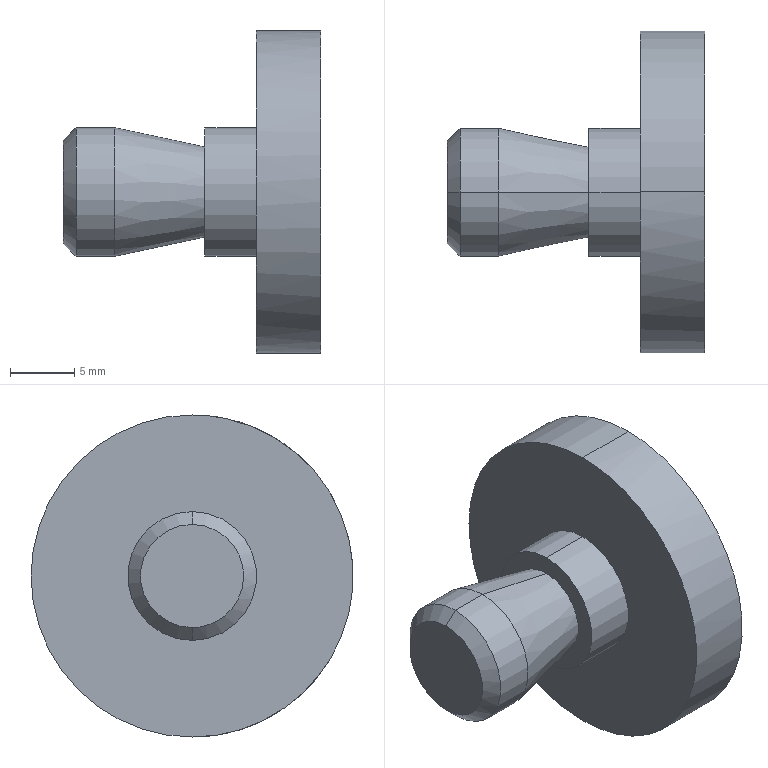Part | STEP file | Positioning_id1786_x_t | 1 solid | 14 faces | box 20 x 25 x 25 mm | volume 3469 mm3 | cylinder 6 | plane 4 | cone 4 | commonest cylinder face diameters 10 x4 25 x2
STEP:
#1=CARTESIAN_POINT('',(0.,0.,0.));
#2=DIRECTION('',(0.,0.,1.));
#3=DIRECTION('',(1.,0.,0.));
#4=AXIS2_PLACEMENT_3D('',#1,#2,#3);
#5=CARTESIAN_POINT('',(-664.,472.5,257.497));
#6=VERTEX_POINT('',#5);
#7=CARTESIAN_POINT('',(-659.,472.5,257.497));
#8=VERTEX_POINT('',#7);
#9=CARTESIAN_POINT('',(-664.,472.5,257.497));
#10=DIRECTION('',(1.,0.,0.));
#11=VECTOR('',#10,1.);
#12=LINE('',#9,#11);
#13=CARTESIAN_POINT('',(-669.,472.5,269.997));
#14=DIRECTION('',(-1.,0.,0.));
#15=DIRECTION('',(0.,0.,-1.));
#16=AXIS2_PLACEMENT_3D('',#13,#14,#15);
#17=CYLINDRICAL_SURFACE('',#16,12.5);
#18=CARTESIAN_POINT('',(6.283,-5.));
#19=DIRECTION('',(0.,-1.));
#20=VECTOR('',#19,1.);
#21=LINE('',#18,#20);
#22=(GEOMETRIC_REPRESENTATION_CONTEXT(2)PARAMETRIC_REPRESENTATION_CONTEXT()REPRESENTATION_CONTEXT('',''));
#23=DEFINITIONAL_REPRESENTATION('',(#21),#22);
#24=PCURVE('',#17,#23);
#25=CARTESIAN_POINT('',(-669.,472.5,269.997));
#26=DIRECTION('',(-1.,0.,0.));
#27=DIRECTION('',(0.,0.,-1.));
#28=AXIS2_PLACEMENT_3D('',#25,#26,#27);
#29=CYLINDRICAL_SURFACE('',#28,12.5);
#30=CARTESIAN_POINT('',(0.,-5.));
#31=DIRECTION('',(0.,-1.));
#32=VECTOR('',#31,1.);
#33=LINE('',#30,#32);
#34=(GEOMETRIC_REPRESENTATION_CONTEXT(2)PARAMETRIC_REPRESENTATION_CONTEXT()REPRESENTATION_CONTEXT('',''));
#35=DEFINITIONAL_REPRESENTATION('',(#33),#34);
#36=PCURVE('',#29,#35);
#37=SURFACE_CURVE('',#12,(#24,#36),.PCURVE_S1.);
#38=EDGE_CURVE('',#6,#8,#37,.T.);
#39=ORIENTED_EDGE('',*,*,#38,.F.);
#40=CARTESIAN_POINT('',(-664.,472.5,282.497));
#41=VERTEX_POINT('',#40);
#42=CARTESIAN_POINT('',(-664.,472.5,269.997));
#43=DIRECTION('',(-1.,0.,0.));
#44=DIRECTION('',(0.,-1.,0.));
#45=AXIS2_PLACEMENT_3D('',#42,#43,#44);
#46=CIRCLE('',#45,12.5);
#47=CARTESIAN_POINT('',(1.571,-5.));
#48=DIRECTION('',(1.,0.));
#49=VECTOR('',#48,1.);
#50=LINE('',#47,#49);
#51=(GEOMETRIC_REPRESENTATION_CONTEXT(2)PARAMETRIC_REPRESENTATION_CONTEXT()REPRESENTATION_CONTEXT('',''));
#52=DEFINITIONAL_REPRESENTATION('',(#50),#51);
#53=PCURVE('',#17,#52);
#54=CARTESIAN_POINT('',(-664.,472.5,269.997));
#55=DIRECTION('',(-1.,0.,0.));
#56=DIRECTION('',(0.,0.,1.));
#57=AXIS2_PLACEMENT_3D('',#54,#55,#56);
#58=PLANE('',#57);
#59=CARTESIAN_POINT('',(0.,0.));
#60=DIRECTION('',(0.,-1.));
#61=AXIS2_PLACEMENT_2D('',#59,#60);
#62=CIRCLE('',#61,12.5);
#63=(GEOMETRIC_REPRESENTATION_CONTEXT(2)PARAMETRIC_REPRESENTATION_CONTEXT()REPRESENTATION_CONTEXT('',''));
#64=DEFINITIONAL_REPRESENTATION('',(#62),#63);
#65=PCURVE('',#58,#64);
#66=SURFACE_CURVE('',#46,(#53,#65),.PCURVE_S1.);
#67=EDGE_CURVE('',#41,#6,#66,.T.);
#68=ORIENTED_EDGE('',*,*,#67,.F.);
#69=CARTESIAN_POINT('',(-659.,472.5,282.497));
#70=VERTEX_POINT('',#69);
#71=CARTESIAN_POINT('',(-664.,472.5,282.497));
#72=DIRECTION('',(-1.,0.,0.));
#73=VECTOR('',#72,1.);
#74=LINE('',#71,#73);
#75=CARTESIAN_POINT('',(3.142,-5.));
#76=DIRECTION('',(0.,1.));
#77=VECTOR('',#76,1.);
#78=LINE('',#75,#77);
#79=(GEOMETRIC_REPRESENTATION_CONTEXT(2)PARAMETRIC_REPRESENTATION_CONTEXT()REPRESENTATION_CONTEXT('',''));
#80=DEFINITIONAL_REPRESENTATION('',(#78),#79);
#81=PCURVE('',#17,#80);
#82=CARTESIAN_POINT('',(3.142,-5.));
#83=DIRECTION('',(0.,1.));
#84=VECTOR('',#83,1.);
#85=LINE('',#82,#84);
#86=(GEOMETRIC_REPRESENTATION_CONTEXT(2)PARAMETRIC_REPRESENTATION_CONTEXT()REPRESENTATION_CONTEXT('',''));
#87=DEFINITIONAL_REPRESENTATION('',(#85),#86);
#88=PCURVE('',#29,#87);
#89=SURFACE_CURVE('',#74,(#81,#88),.PCURVE_S1.);
#90=EDGE_CURVE('',#70,#41,#89,.T.);
#91=ORIENTED_EDGE('',*,*,#90,.F.);
#92=CARTESIAN_POINT('',(-659.,472.5,269.997));
#93=DIRECTION('',(1.,0.,0.));
#94=DIRECTION('',(0.,-1.,0.));
#95=AXIS2_PLACEMENT_3D('',#92,#93,#94);
#96=CIRCLE('',#95,12.5);
#97=CARTESIAN_POINT('',(7.854,-10.));
#98=DIRECTION('',(-1.,0.));
#99=VECTOR('',#98,1.);
#100=LINE('',#97,#99);
#101=(GEOMETRIC_REPRESENTATION_CONTEXT(2)PARAMETRIC_REPRESENTATION_CONTEXT()REPRESENTATION_CONTEXT('',''));
#102=DEFINITIONAL_REPRESENTATION('',(#100),#101);
#103=PCURVE('',#17,#102);
#104=CARTESIAN_POINT('',(-659.,472.5,269.997));
#105=DIRECTION('',(1.,0.,0.));
#106=DIRECTION('',(0.,0.,-1.));
#107=AXIS2_PLACEMENT_3D('',#104,#105,#106);
#108=PLANE('',#107);
#109=CARTESIAN_POINT('',(0.,0.));
#110=DIRECTION('',(0.,-1.));
#111=AXIS2_PLACEMENT_2D('',#109,#110);
#112=CIRCLE('',#111,12.5);
#113=(GEOMETRIC_REPRESENTATION_CONTEXT(2)PARAMETRIC_REPRESENTATION_CONTEXT()REPRESENTATION_CONTEXT('',''));
#114=DEFINITIONAL_REPRESENTATION('',(#112),#113);
#115=PCURVE('',#108,#114);
#116=SURFACE_CURVE('',#96,(#103,#115),.PCURVE_S1.);
#117=EDGE_CURVE('',#8,#70,#116,.T.);
#118=ORIENTED_EDGE('',*,*,#117,.F.);
#119=EDGE_LOOP('',(#39,#68,#91,#118));
#120=FACE_BOUND('',#119,.T.);
#121=ADVANCED_FACE('',(#120),#17,.T.);
#122=CARTESIAN_POINT('',(-664.,472.5,274.997));
#123=VERTEX_POINT('',#122);
#124=CARTESIAN_POINT('',(-664.,472.5,264.997));
#125=VERTEX_POINT('',#124);
#126=CARTESIAN_POINT('',(-664.,472.5,269.997));
#127=DIRECTION('',(-1.,0.,0.));
#128=DIRECTION('',(0.,0.,1.));
#129=AXIS2_PLACEMENT_3D('',#126,#127,#128);
#130=CIRCLE('',#129,5.);
#131=CARTESIAN_POINT('',(0.,0.));
#132=DIRECTION('',(1.,0.));
#133=AXIS2_PLACEMENT_2D('',#131,#132);
#134=CIRCLE('',#133,5.);
#135=(GEOMETRIC_REPRESENTATION_CONTEXT(2)PARAMETRIC_REPRESENTATION_CONTEXT()REPRESENTATION_CONTEXT('',''));
#136=DEFINITIONAL_REPRESENTATION('',(#134),#135);
#137=PCURVE('',#58,#136);
#138=CARTESIAN_POINT('',(-669.,472.5,269.997));
#139=DIRECTION('',(-1.,0.,0.));
#140=DIRECTION('',(0.,0.,-1.));
#141=AXIS2_PLACEMENT_3D('',#138,#139,#140);
#142=CYLINDRICAL_SURFACE('',#141,5.);
#143=CARTESIAN_POINT('',(3.142,-5.));
#144=DIRECTION('',(1.,0.));
#145=VECTOR('',#144,1.);
#146=LINE('',#143,#145);
#147=(GEOMETRIC_REPRESENTATION_CONTEXT(2)PARAMETRIC_REPRESENTATION_CONTEXT()REPRESENTATION_CONTEXT('',''));
#148=DEFINITIONAL_REPRESENTATION('',(#146),#147);
#149=PCURVE('',#142,#148);
#150=SURFACE_CURVE('',#130,(#137,#149),.PCURVE_S1.);
#151=EDGE_CURVE('',#123,#125,#150,.T.);
#152=ORIENTED_EDGE('',*,*,#151,.F.);
#153=CARTESIAN_POINT('',(-664.,472.5,269.997));
#154=DIRECTION('',(-1.,0.,0.));
#155=DIRECTION('',(0.,0.,-1.));
#156=AXIS2_PLACEMENT_3D('',#153,#154,#155);
#157=CIRCLE('',#156,5.);
#158=CARTESIAN_POINT('',(0.,0.));
#159=DIRECTION('',(-1.,0.));
#160=AXIS2_PLACEMENT_2D('',#158,#159);
#161=CIRCLE('',#160,5.);
#162=(GEOMETRIC_REPRESENTATION_CONTEXT(2)PARAMETRIC_REPRESENTATION_CONTEXT()REPRESENTATION_CONTEXT('',''));
#163=DEFINITIONAL_REPRESENTATION('',(#161),#162);
#164=PCURVE('',#58,#163);
#165=CARTESIAN_POINT('',(-669.,472.5,269.997));
#166=DIRECTION('',(-1.,0.,0.));
#167=DIRECTION('',(0.,0.,-1.));
#168=AXIS2_PLACEMENT_3D('',#165,#166,#167);
#169=CYLINDRICAL_SURFACE('',#168,5.);
#170=CARTESIAN_POINT('',(0.,-5.));
#171=DIRECTION('',(1.,0.));
#172=VECTOR('',#171,1.);
#173=LINE('',#170,#172);
#174=(GEOMETRIC_REPRESENTATION_CONTEXT(2)PARAMETRIC_REPRESENTATION_CONTEXT()REPRESENTATION_CONTEXT('',''));
#175=DEFINITIONAL_REPRESENTATION('',(#173),#174);
#176=PCURVE('',#169,#175);
#177=SURFACE_CURVE('',#157,(#164,#176),.PCURVE_S1.);
#178=EDGE_CURVE('',#125,#123,#177,.T.);
#179=ORIENTED_EDGE('',*,*,#178,.F.);
#180=EDGE_LOOP('',(#152,#179));
#181=FACE_BOUND('',#180,.T.);
#182=ORIENTED_EDGE('',*,*,#67,.T.);
#183=CARTESIAN_POINT('',(-664.,472.5,257.497));
#184=CARTESIAN_POINT('',(-664.,460.,257.497));
#185=CARTESIAN_POINT('',(-664.,453.75,269.997));
#186=CARTESIAN_POINT('',(-664.,460.,282.497));
#187=CARTESIAN_POINT('',(-664.,472.5,282.497));
#188=(BOUNDED_CURVE()B_SPLINE_CURVE(4,(#183,#184,#185,#186,#187),.UNSPECIFIED.,.F.,.F.)B_SPLINE_CURVE_WITH_KNOTS((5,5),(0.,1.),.PIECEWISE_BEZIER_KNOTS.)CURVE()GEOMETRIC_REPRESENTATION_ITEM()RATIONAL_B_SPLINE_CURVE((1.,0.7071,0.6667,0.7071,1.))REPRESENTATION_ITEM(''));
#189=CARTESIAN_POINT('',(-12.5,0.));
#190=CARTESIAN_POINT('',(-12.5,-12.5));
#191=CARTESIAN_POINT('',(0.,-18.75));
#192=CARTESIAN_POINT('',(12.5,-12.5));
#193=CARTESIAN_POINT('',(12.5,0.));
#194=(BOUNDED_CURVE()B_SPLINE_CURVE(4,(#189,#190,#191,#192,#193),.UNSPECIFIED.,.F.,.F.)B_SPLINE_CURVE_WITH_KNOTS((5,5),(0.,1.),.PIECEWISE_BEZIER_KNOTS.)CURVE()GEOMETRIC_REPRESENTATION_ITEM()RATIONAL_B_SPLINE_CURVE((1.,0.7071,0.6667,0.7071,1.))REPRESENTATION_ITEM(''));
#195=(GEOMETRIC_REPRESENTATION_CONTEXT(2)PARAMETRIC_REPRESENTATION_CONTEXT()REPRESENTATION_CONTEXT('',''));
#196=DEFINITIONAL_REPRESENTATION('',(#194),#195);
#197=PCURVE('',#58,#196);
#198=CARTESIAN_POINT('',(0.,-5.));
#199=CARTESIAN_POINT('',(0.04285,-5.));
#200=CARTESIAN_POINT('',(0.1297,-5.));
#201=CARTESIAN_POINT('',(0.2633,-5.));
#202=CARTESIAN_POINT('',(0.3999,-5.));
#203=CARTESIAN_POINT('',(0.5394,-5.));
#204=CARTESIAN_POINT('',(0.6816,-5.));
#205=CARTESIAN_POINT('',(0.8261,-5.));
#206=CARTESIAN_POINT('',(0.9725,-5.));
#207=CARTESIAN_POINT('',(1.121,-5.));
#208=CARTESIAN_POINT('',(1.27,-5.));
#209=CARTESIAN_POINT('',(1.42,-5.));
#210=CARTESIAN_POINT('',(1.571,-5.));
#211=CARTESIAN_POINT('',(1.721,-5.));
#212=CARTESIAN_POINT('',(1.872,-5.));
#213=CARTESIAN_POINT('',(2.021,-5.));
#214=CARTESIAN_POINT('',(2.169,-5.));
#215=CARTESIAN_POINT('',(2.316,-5.));
#216=CARTESIAN_POINT('',(2.46,-5.));
#217=CARTESIAN_POINT('',(2.602,-5.));
#218=CARTESIAN_POINT('',(2.742,-5.));
#219=CARTESIAN_POINT('',(2.878,-5.));
#220=CARTESIAN_POINT('',(3.012,-5.));
#221=CARTESIAN_POINT('',(3.099,-5.));
#222=CARTESIAN_POINT('',(3.142,-5.));
#223=B_SPLINE_CURVE_WITH_KNOTS('',3,(#198,#199,#200,#201,#202,#203,#204,#205,#206,#207,#208,#209,#210,#211,#212,#213,#214,#215,#216,#217,#218,#219,#220,#221,#222),.UNSPECIFIED.,.F.,.F.,(4,1,1,1,1,1,1,1,1,1,1,1,1,1,1,1,1,1,1,1,1,1,4),(0.,0.04545,0.09091,0.1364,0.1818,0.2273,0.2727,0.3182,0.3636,0.4091,0.4545,0.5,0.5455,0.5909,0.6364,0.6818,0.7273,0.7727,0.8182,0.8636,0.9091,0.9545,1.),.QUASI_UNIFORM_KNOTS.);
#224=(GEOMETRIC_REPRESENTATION_CONTEXT(2)PARAMETRIC_REPRESENTATION_CONTEXT()REPRESENTATION_CONTEXT('',''));
#225=DEFINITIONAL_REPRESENTATION('',(#223),#224);
#226=PCURVE('',#29,#225);
#227=SURFACE_CURVE('',#188,(#197,#226),.PCURVE_S1.);
#228=EDGE_CURVE('',#6,#41,#227,.T.);
#229=ORIENTED_EDGE('',*,*,#228,.T.);
#230=EDGE_LOOP('',(#182,#229));
#231=FACE_BOUND('',#230,.T.);
#232=ADVANCED_FACE('',(#181,#231),#58,.T.);
#233=CARTESIAN_POINT('',(-659.,472.5,282.497));
#234=CARTESIAN_POINT('',(-659.,460.,282.497));
#235=CARTESIAN_POINT('',(-659.,453.75,269.997));
#236=CARTESIAN_POINT('',(-659.,460.,257.497));
#237=CARTESIAN_POINT('',(-659.,472.5,257.497));
#238=(BOUNDED_CURVE()B_SPLINE_CURVE(4,(#233,#234,#235,#236,#237),.UNSPECIFIED.,.F.,.F.)B_SPLINE_CURVE_WITH_KNOTS((5,5),(0.,1.),.PIECEWISE_BEZIER_KNOTS.)CURVE()GEOMETRIC_REPRESENTATION_ITEM()RATIONAL_B_SPLINE_CURVE((1.,0.7071,0.6667,0.7071,1.))REPRESENTATION_ITEM(''));
#239=CARTESIAN_POINT('',(-12.5,0.));
#240=CARTESIAN_POINT('',(-12.5,-12.5));
#241=CARTESIAN_POINT('',(0.,-18.75));
#242=CARTESIAN_POINT('',(12.5,-12.5));
#243=CARTESIAN_POINT('',(12.5,0.));
#244=(BOUNDED_CURVE()B_SPLINE_CURVE(4,(#239,#240,#241,#242,#243),.UNSPECIFIED.,.F.,.F.)B_SPLINE_CURVE_WITH_KNOTS((5,5),(0.,1.),.PIECEWISE_BEZIER_KNOTS.)CURVE()GEOMETRIC_REPRESENTATION_ITEM()RATIONAL_B_SPLINE_CURVE((1.,0.7071,0.6667,0.7071,1.))REPRESENTATION_ITEM(''));
#245=(GEOMETRIC_REPRESENTATION_CONTEXT(2)PARAMETRIC_REPRESENTATION_CONTEXT()REPRESENTATION_CONTEXT('',''));
#246=DEFINITIONAL_REPRESENTATION('',(#244),#245);
#247=PCURVE('',#108,#246);
#248=CARTESIAN_POINT('',(3.142,-10.));
#249=CARTESIAN_POINT('',(3.099,-10.));
#250=CARTESIAN_POINT('',(3.012,-10.));
#251=CARTESIAN_POINT('',(2.878,-10.));
#252=CARTESIAN_POINT('',(2.742,-10.));
#253=CARTESIAN_POINT('',(2.602,-10.));
#254=CARTESIAN_POINT('',(2.46,-10.));
#255=CARTESIAN_POINT('',(2.316,-10.));
#256=CARTESIAN_POINT('',(2.169,-10.));
#257=CARTESIAN_POINT('',(2.021,-10.));
#258=CARTESIAN_POINT('',(1.872,-10.));
#259=CARTESIAN_POINT('',(1.721,-10.));
#260=CARTESIAN_POINT('',(1.571,-10.));
#261=CARTESIAN_POINT('',(1.42,-10.));
#262=CARTESIAN_POINT('',(1.27,-10.));
#263=CARTESIAN_POINT('',(1.121,-10.));
#264=CARTESIAN_POINT('',(0.9725,-10.));
#265=CARTESIAN_POINT('',(0.8261,-10.));
#266=CARTESIAN_POINT('',(0.6816,-10.));
#267=CARTESIAN_POINT('',(0.5394,-10.));
#268=CARTESIAN_POINT('',(0.3999,-10.));
#269=CARTESIAN_POINT('',(0.2633,-10.));
#270=CARTESIAN_POINT('',(0.1297,-10.));
#271=CARTESIAN_POINT('',(0.04285,-10.));
#272=CARTESIAN_POINT('',(0.,-10.));
#273=B_SPLINE_CURVE_WITH_KNOTS('',3,(#248,#249,#250,#251,#252,#253,#254,#255,#256,#257,#258,#259,#260,#261,#262,#263,#264,#265,#266,#267,#268,#269,#270,#271,#272),.UNSPECIFIED.,.F.,.F.,(4,1,1,1,1,1,1,1,1,1,1,1,1,1,1,1,1,1,1,1,1,1,4),(0.,0.04545,0.09091,0.1364,0.1818,0.2273,0.2727,0.3182,0.3636,0.4091,0.4545,0.5,0.5455,0.5909,0.6364,0.6818,0.7273,0.7727,0.8182,0.8636,0.9091,0.9545,1.),.QUASI_UNIFORM_KNOTS.);
#274=(GEOMETRIC_REPRESENTATION_CONTEXT(2)PARAMETRIC_REPRESENTATION_CONTEXT()REPRESENTATION_CONTEXT('',''));
#275=DEFINITIONAL_REPRESENTATION('',(#273),#274);
#276=PCURVE('',#29,#275);
#277=SURFACE_CURVE('',#238,(#247,#276),.PCURVE_S1.);
#278=EDGE_CURVE('',#70,#8,#277,.T.);
#279=ORIENTED_EDGE('',*,*,#278,.T.);
#280=ORIENTED_EDGE('',*,*,#117,.T.);
#281=EDGE_LOOP('',(#279,#280));
#282=FACE_BOUND('',#281,.T.);
#283=ADVANCED_FACE('',(#282),#108,.T.);
#284=CARTESIAN_POINT('',(-668.,472.5,266.497));
#285=VERTEX_POINT('',#284);
#286=CARTESIAN_POINT('',(-668.,472.5,273.497));
#287=VERTEX_POINT('',#286);
#288=CARTESIAN_POINT('',(-668.,472.5,269.997));
#289=DIRECTION('',(-1.,0.,0.));
#290=DIRECTION('',(0.,0.,-1.));
#291=AXIS2_PLACEMENT_3D('',#288,#289,#290);
#292=CIRCLE('',#291,3.5);
#293=CARTESIAN_POINT('',(-668.,472.5,269.997));
#294=DIRECTION('',(1.,0.,0.));
#295=DIRECTION('',(0.,0.,-1.));
#296=AXIS2_PLACEMENT_3D('',#293,#294,#295);
#297=PLANE('',#296);
#298=CARTESIAN_POINT('',(3.5,0.));
#299=CARTESIAN_POINT('',(3.5,-6.062));
#300=CARTESIAN_POINT('',(-1.75,-3.031));
#301=CARTESIAN_POINT('',(-7.,0.));
#302=CARTESIAN_POINT('',(-1.75,3.031));
#303=CARTESIAN_POINT('',(3.5,6.062));
#304=CARTESIAN_POINT('',(3.5,0.));
#305=(BOUNDED_CURVE()B_SPLINE_CURVE(2,(#298,#299,#300,#301,#302,#303,#304),.UNSPECIFIED.,.T.,.F.)B_SPLINE_CURVE_WITH_KNOTS((1,2,2,2,2,1),(-2.094,0.,2.094,4.189,6.283,8.378),.UNSPECIFIED.)CURVE()GEOMETRIC_REPRESENTATION_ITEM()RATIONAL_B_SPLINE_CURVE((1.,0.5,1.,0.5,1.,0.5,1.))REPRESENTATION_ITEM(''));
#306=(GEOMETRIC_REPRESENTATION_CONTEXT(2)PARAMETRIC_REPRESENTATION_CONTEXT()REPRESENTATION_CONTEXT('',''));
#307=DEFINITIONAL_REPRESENTATION('',(#305),#306);
#308=PCURVE('',#297,#307);
#309=CARTESIAN_POINT('',(-675.,472.5,269.997));
#310=DIRECTION('',(-1.,0.,0.));
#311=DIRECTION('',(0.,0.,1.));
#312=AXIS2_PLACEMENT_3D('',#309,#310,#311);
#313=CONICAL_SURFACE('',#312,5.,0.2111);
#314=CARTESIAN_POINT('',(3.142,-7.));
#315=DIRECTION('',(1.,0.));
#316=VECTOR('',#315,1.);
#317=LINE('',#314,#316);
#318=(GEOMETRIC_REPRESENTATION_CONTEXT(2)PARAMETRIC_REPRESENTATION_CONTEXT()REPRESENTATION_CONTEXT('',''));
#319=DEFINITIONAL_REPRESENTATION('',(#317),#318);
#320=PCURVE('',#313,#319);
#321=SURFACE_CURVE('',#292,(#308,#320),.PCURVE_S1.);
#322=EDGE_CURVE('',#285,#287,#321,.T.);
#323=ORIENTED_EDGE('',*,*,#322,.F.);
#324=CARTESIAN_POINT('',(-668.,472.5,269.997));
#325=DIRECTION('',(-1.,0.,0.));
#326=DIRECTION('',(0.,0.,1.));
#327=AXIS2_PLACEMENT_3D('',#324,#325,#326);
#328=CIRCLE('',#327,3.5);
#329=CARTESIAN_POINT('',(-3.5,0.));
#330=CARTESIAN_POINT('',(-3.5,6.062));
#331=CARTESIAN_POINT('',(1.75,3.031));
#332=CARTESIAN_POINT('',(7.,0.));
#333=CARTESIAN_POINT('',(1.75,-3.031));
#334=CARTESIAN_POINT('',(-3.5,-6.062));
#335=CARTESIAN_POINT('',(-3.5,0.));
#336=(BOUNDED_CURVE()B_SPLINE_CURVE(2,(#329,#330,#331,#332,#333,#334,#335),.UNSPECIFIED.,.T.,.F.)B_SPLINE_CURVE_WITH_KNOTS((1,2,2,2,2,1),(-2.094,0.,2.094,4.189,6.283,8.378),.UNSPECIFIED.)CURVE()GEOMETRIC_REPRESENTATION_ITEM()RATIONAL_B_SPLINE_CURVE((1.,0.5,1.,0.5,1.,0.5,1.))REPRESENTATION_ITEM(''));
#337=(GEOMETRIC_REPRESENTATION_CONTEXT(2)PARAMETRIC_REPRESENTATION_CONTEXT()REPRESENTATION_CONTEXT('',''));
#338=DEFINITIONAL_REPRESENTATION('',(#336),#337);
#339=PCURVE('',#297,#338);
#340=CARTESIAN_POINT('',(-675.,472.5,269.997));
#341=DIRECTION('',(-1.,0.,0.));
#342=DIRECTION('',(0.,0.,1.));
#343=AXIS2_PLACEMENT_3D('',#340,#341,#342);
#344=CONICAL_SURFACE('',#343,5.,0.2111);
#345=CARTESIAN_POINT('',(0.,-7.));
#346=DIRECTION('',(1.,0.));
#347=VECTOR('',#346,1.);
#348=LINE('',#345,#347);
#349=(GEOMETRIC_REPRESENTATION_CONTEXT(2)PARAMETRIC_REPRESENTATION_CONTEXT()REPRESENTATION_CONTEXT('',''));
#350=DEFINITIONAL_REPRESENTATION('',(#348),#349);
#351=PCURVE('',#344,#350);
#352=SURFACE_CURVE('',#328,(#339,#351),.PCURVE_S1.);
#353=EDGE_CURVE('',#287,#285,#352,.T.);
#354=ORIENTED_EDGE('',*,*,#353,.F.);
#355=EDGE_LOOP('',(#323,#354));
#356=FACE_BOUND('',#355,.T.);
#357=CARTESIAN_POINT('',(-668.,472.5,274.997));
#358=VERTEX_POINT('',#357);
#359=CARTESIAN_POINT('',(-668.,472.5,264.997));
#360=VERTEX_POINT('',#359);
#361=CARTESIAN_POINT('',(-668.,472.5,269.997));
#362=DIRECTION('',(1.,0.,0.));
#363=DIRECTION('',(0.,0.,1.));
#364=AXIS2_PLACEMENT_3D('',#361,#362,#363);
#365=CIRCLE('',#364,5.);
#366=CARTESIAN_POINT('',(0.,0.));
#367=DIRECTION('',(-1.,0.));
#368=AXIS2_PLACEMENT_2D('',#366,#367);
#369=CIRCLE('',#368,5.);
#370=(GEOMETRIC_REPRESENTATION_CONTEXT(2)PARAMETRIC_REPRESENTATION_CONTEXT()REPRESENTATION_CONTEXT('',''));
#371=DEFINITIONAL_REPRESENTATION('',(#369),#370);
#372=PCURVE('',#297,#371);
#373=CARTESIAN_POINT('',(3.142,-1.));
#374=DIRECTION('',(-1.,0.));
#375=VECTOR('',#374,1.);
#376=LINE('',#373,#375);
#377=(GEOMETRIC_REPRESENTATION_CONTEXT(2)PARAMETRIC_REPRESENTATION_CONTEXT()REPRESENTATION_CONTEXT('',''));
#378=DEFINITIONAL_REPRESENTATION('',(#376),#377);
#379=PCURVE('',#169,#378);
#380=SURFACE_CURVE('',#365,(#372,#379),.PCURVE_S1.);
#381=EDGE_CURVE('',#358,#360,#380,.T.);
#382=ORIENTED_EDGE('',*,*,#381,.F.);
#383=CARTESIAN_POINT('',(-668.,472.5,269.997));
#384=DIRECTION('',(1.,0.,0.));
#385=DIRECTION('',(0.,0.,-1.));
#386=AXIS2_PLACEMENT_3D('',#383,#384,#385);
#387=CIRCLE('',#386,5.);
#388=CARTESIAN_POINT('',(0.,0.));
#389=DIRECTION('',(1.,0.));
#390=AXIS2_PLACEMENT_2D('',#388,#389);
#391=CIRCLE('',#390,5.);
#392=(GEOMETRIC_REPRESENTATION_CONTEXT(2)PARAMETRIC_REPRESENTATION_CONTEXT()REPRESENTATION_CONTEXT('',''));
#393=DEFINITIONAL_REPRESENTATION('',(#391),#392);
#394=PCURVE('',#297,#393);
#395=CARTESIAN_POINT('',(6.283,-1.));
#396=DIRECTION('',(-1.,0.));
#397=VECTOR('',#396,1.);
#398=LINE('',#395,#397);
#399=(GEOMETRIC_REPRESENTATION_CONTEXT(2)PARAMETRIC_REPRESENTATION_CONTEXT()REPRESENTATION_CONTEXT('',''));
#400=DEFINITIONAL_REPRESENTATION('',(#398),#399);
#401=PCURVE('',#142,#400);
#402=SURFACE_CURVE('',#387,(#394,#401),.PCURVE_S1.);
#403=EDGE_CURVE('',#360,#358,#402,.T.);
#404=ORIENTED_EDGE('',*,*,#403,.F.);
#405=EDGE_LOOP('',(#382,#404));
#406=FACE_BOUND('',#405,.T.);
#407=ADVANCED_FACE('',(#356,#406),#297,.F.);
#408=CARTESIAN_POINT('',(-668.,472.5,264.997));
#409=DIRECTION('',(1.,0.,0.));
#410=VECTOR('',#409,1.);
#411=LINE('',#408,#410);
#412=CARTESIAN_POINT('',(6.283,-1.));
#413=DIRECTION('',(0.,-1.));
#414=VECTOR('',#413,1.);
#415=LINE('',#412,#414);
#416=(GEOMETRIC_REPRESENTATION_CONTEXT(2)PARAMETRIC_REPRESENTATION_CONTEXT()REPRESENTATION_CONTEXT('',''));
#417=DEFINITIONAL_REPRESENTATION('',(#415),#416);
#418=PCURVE('',#142,#417);
#419=CARTESIAN_POINT('',(0.,-1.));
#420=DIRECTION('',(0.,-1.));
#421=VECTOR('',#420,1.);
#422=LINE('',#419,#421);
#423=(GEOMETRIC_REPRESENTATION_CONTEXT(2)PARAMETRIC_REPRESENTATION_CONTEXT()REPRESENTATION_CONTEXT('',''));
#424=DEFINITIONAL_REPRESENTATION('',(#422),#423);
#425=PCURVE('',#169,#424);
#426=SURFACE_CURVE('',#411,(#418,#425),.PCURVE_S1.);
#427=EDGE_CURVE('',#360,#125,#426,.T.);
#428=ORIENTED_EDGE('',*,*,#427,.F.);
#429=ORIENTED_EDGE('',*,*,#403,.T.);
#430=CARTESIAN_POINT('',(-668.,472.5,274.997));
#431=DIRECTION('',(-1.,0.,0.));
#432=VECTOR('',#431,1.);
#433=LINE('',#430,#432);
#434=CARTESIAN_POINT('',(3.142,-1.));
#435=DIRECTION('',(0.,1.));
#436=VECTOR('',#435,1.);
#437=LINE('',#434,#436);
#438=(GEOMETRIC_REPRESENTATION_CONTEXT(2)PARAMETRIC_REPRESENTATION_CONTEXT()REPRESENTATION_CONTEXT('',''));
#439=DEFINITIONAL_REPRESENTATION('',(#437),#438);
#440=PCURVE('',#142,#439);
#441=CARTESIAN_POINT('',(3.142,-1.));
#442=DIRECTION('',(0.,1.));
#443=VECTOR('',#442,1.);
#444=LINE('',#441,#443);
#445=(GEOMETRIC_REPRESENTATION_CONTEXT(2)PARAMETRIC_REPRESENTATION_CONTEXT()REPRESENTATION_CONTEXT('',''));
#446=DEFINITIONAL_REPRESENTATION('',(#444),#445);
#447=PCURVE('',#169,#446);
#448=SURFACE_CURVE('',#433,(#440,#447),.PCURVE_S1.);
#449=EDGE_CURVE('',#123,#358,#448,.T.);
#450=ORIENTED_EDGE('',*,*,#449,.F.);
#451=ORIENTED_EDGE('',*,*,#151,.T.);
#452=EDGE_LOOP('',(#428,#429,#450,#451));
#453=FACE_BOUND('',#452,.T.);
#454=ADVANCED_FACE('',(#453),#142,.T.);
#455=CARTESIAN_POINT('',(-675.,472.5,274.997));
#456=VERTEX_POINT('',#455);
#457=CARTESIAN_POINT('',(-668.,472.5,273.497));
#458=DIRECTION('',(-0.9778,0.,0.2095));
#459=VECTOR('',#458,1.);
#460=LINE('',#457,#459);
#461=CARTESIAN_POINT('',(0.,-7.));
#462=DIRECTION('',(0.,1.));
#463=VECTOR('',#462,1.);
#464=LINE('',#461,#463);
#465=(GEOMETRIC_REPRESENTATION_CONTEXT(2)PARAMETRIC_REPRESENTATION_CONTEXT()REPRESENTATION_CONTEXT('',''));
#466=DEFINITIONAL_REPRESENTATION('',(#464),#465);
#467=PCURVE('',#344,#466);
#468=CARTESIAN_POINT('',(6.283,-7.));
#469=DIRECTION('',(0.,1.));
#470=VECTOR('',#469,1.);
#471=LINE('',#468,#470);
#472=(GEOMETRIC_REPRESENTATION_CONTEXT(2)PARAMETRIC_REPRESENTATION_CONTEXT()REPRESENTATION_CONTEXT('',''));
#473=DEFINITIONAL_REPRESENTATION('',(#471),#472);
#474=PCURVE('',#313,#473);
#475=SURFACE_CURVE('',#460,(#467,#474),.PCURVE_S1.);
#476=EDGE_CURVE('',#287,#456,#475,.T.);
#477=ORIENTED_EDGE('',*,*,#476,.F.);
#478=ORIENTED_EDGE('',*,*,#353,.T.);
#479=CARTESIAN_POINT('',(-675.,472.5,264.997));
#480=VERTEX_POINT('',#479);
#481=CARTESIAN_POINT('',(-668.,472.5,266.497));
#482=DIRECTION('',(0.9778,0.,0.2095));
#483=VECTOR('',#482,1.);
#484=LINE('',#481,#483);
#485=CARTESIAN_POINT('',(3.142,-7.));
#486=DIRECTION('',(0.,-1.));
#487=VECTOR('',#486,1.);
#488=LINE('',#485,#487);
#489=(GEOMETRIC_REPRESENTATION_CONTEXT(2)PARAMETRIC_REPRESENTATION_CONTEXT()REPRESENTATION_CONTEXT('',''));
#490=DEFINITIONAL_REPRESENTATION('',(#488),#489);
#491=PCURVE('',#344,#490);
#492=CARTESIAN_POINT('',(3.142,-7.));
#493=DIRECTION('',(0.,-1.));
#494=VECTOR('',#493,1.);
#495=LINE('',#492,#494);
#496=(GEOMETRIC_REPRESENTATION_CONTEXT(2)PARAMETRIC_REPRESENTATION_CONTEXT()REPRESENTATION_CONTEXT('',''));
#497=DEFINITIONAL_REPRESENTATION('',(#495),#496);
#498=PCURVE('',#313,#497);
#499=SURFACE_CURVE('',#484,(#491,#498),.PCURVE_S1.);
#500=EDGE_CURVE('',#480,#285,#499,.T.);
#501=ORIENTED_EDGE('',*,*,#500,.F.);
#502=CARTESIAN_POINT('',(-675.,472.5,269.997));
#503=DIRECTION('',(1.,0.,0.));
#504=DIRECTION('',(0.,0.,-1.));
#505=AXIS2_PLACEMENT_3D('',#502,#503,#504);
#506=CIRCLE('',#505,5.);
#507=CARTESIAN_POINT('',(3.142,0.));
#508=DIRECTION('',(-1.,0.));
#509=VECTOR('',#508,1.);
#510=LINE('',#507,#509);
#511=(GEOMETRIC_REPRESENTATION_CONTEXT(2)PARAMETRIC_REPRESENTATION_CONTEXT()REPRESENTATION_CONTEXT('',''));
#512=DEFINITIONAL_REPRESENTATION('',(#510),#511);
#513=PCURVE('',#344,#512);
#514=CARTESIAN_POINT('',(-669.,472.5,269.997));
#515=DIRECTION('',(-1.,0.,0.));
#516=DIRECTION('',(0.,0.,-1.));
#517=AXIS2_PLACEMENT_3D('',#514,#515,#516);
#518=CYLINDRICAL_SURFACE('',#517,5.);
#519=CARTESIAN_POINT('',(6.283,6.));
#520=DIRECTION('',(-1.,0.));
#521=VECTOR('',#520,1.);
#522=LINE('',#519,#521);
#523=(GEOMETRIC_REPRESENTATION_CONTEXT(2)PARAMETRIC_REPRESENTATION_CONTEXT()REPRESENTATION_CONTEXT('',''));
#524=DEFINITIONAL_REPRESENTATION('',(#522),#523);
#525=PCURVE('',#518,#524);
#526=SURFACE_CURVE('',#506,(#513,#525),.PCURVE_S1.);
#527=EDGE_CURVE('',#480,#456,#526,.T.);
#528=ORIENTED_EDGE('',*,*,#527,.T.);
#529=EDGE_LOOP('',(#477,#478,#501,#528));
#530=FACE_BOUND('',#529,.T.);
#531=ADVANCED_FACE('',(#530),#344,.T.);
#532=CARTESIAN_POINT('',(-679.,472.5,265.997));
#533=VERTEX_POINT('',#532);
#534=CARTESIAN_POINT('',(-678.,472.5,264.997));
#535=VERTEX_POINT('',#534);
#536=CARTESIAN_POINT('',(-679.,472.5,265.997));
#537=DIRECTION('',(0.7071,0.,-0.7071));
#538=VECTOR('',#537,1.);
#539=LINE('',#536,#538);
#540=CARTESIAN_POINT('',(-678.,472.5,269.997));
#541=DIRECTION('',(1.,0.,0.));
#542=DIRECTION('',(0.,0.,-1.));
#543=AXIS2_PLACEMENT_3D('',#540,#541,#542);
#544=CONICAL_SURFACE('',#543,5.,0.7854);
#545=CARTESIAN_POINT('',(0.,-1.));
#546=DIRECTION('',(0.,1.));
#547=VECTOR('',#546,1.);
#548=LINE('',#545,#547);
#549=(GEOMETRIC_REPRESENTATION_CONTEXT(2)PARAMETRIC_REPRESENTATION_CONTEXT()REPRESENTATION_CONTEXT('',''));
#550=DEFINITIONAL_REPRESENTATION('',(#548),#549);
#551=PCURVE('',#544,#550);
#552=CARTESIAN_POINT('',(-678.,472.5,269.997));
#553=DIRECTION('',(1.,0.,0.));
#554=DIRECTION('',(0.,0.,-1.));
#555=AXIS2_PLACEMENT_3D('',#552,#553,#554);
#556=CONICAL_SURFACE('',#555,5.,0.7854);
#557=CARTESIAN_POINT('',(6.283,-1.));
#558=DIRECTION('',(0.,1.));
#559=VECTOR('',#558,1.);
#560=LINE('',#557,#559);
#561=(GEOMETRIC_REPRESENTATION_CONTEXT(2)PARAMETRIC_REPRESENTATION_CONTEXT()REPRESENTATION_CONTEXT('',''));
#562=DEFINITIONAL_REPRESENTATION('',(#560),#561);
#563=PCURVE('',#556,#562);
#564=SURFACE_CURVE('',#539,(#551,#563),.PCURVE_S1.);
#565=EDGE_CURVE('',#533,#535,#564,.T.);
#566=ORIENTED_EDGE('',*,*,#565,.F.);
#567=CARTESIAN_POINT('',(-679.,472.5,273.997));
#568=VERTEX_POINT('',#567);
#569=CARTESIAN_POINT('',(-679.,472.5,269.997));
#570=DIRECTION('',(1.,0.,0.));
#571=DIRECTION('',(0.,1.,0.));
#572=AXIS2_PLACEMENT_3D('',#569,#570,#571);
#573=CIRCLE('',#572,4.);
#574=CARTESIAN_POINT('',(-4.712,-1.));
#575=DIRECTION('',(1.,0.));
#576=VECTOR('',#575,1.);
#577=LINE('',#574,#576);
#578=(GEOMETRIC_REPRESENTATION_CONTEXT(2)PARAMETRIC_REPRESENTATION_CONTEXT()REPRESENTATION_CONTEXT('',''));
#579=DEFINITIONAL_REPRESENTATION('',(#577),#578);
#580=PCURVE('',#544,#579);
#581=CARTESIAN_POINT('',(-679.,472.5,269.997));
#582=DIRECTION('',(-1.,0.,0.));
#583=DIRECTION('',(0.,0.,1.));
#584=AXIS2_PLACEMENT_3D('',#581,#582,#583);
#585=PLANE('',#584);
#586=CARTESIAN_POINT('',(0.,4.));
#587=CARTESIAN_POINT('',(6.928,4.));
#588=CARTESIAN_POINT('',(3.464,-2.));
#589=CARTESIAN_POINT('',(0.,-8.));
#590=CARTESIAN_POINT('',(-3.464,-2.));
#591=CARTESIAN_POINT('',(-6.928,4.));
#592=CARTESIAN_POINT('',(0.,4.));
#593=(BOUNDED_CURVE()B_SPLINE_CURVE(2,(#586,#587,#588,#589,#590,#591,#592),.UNSPECIFIED.,.T.,.F.)B_SPLINE_CURVE_WITH_KNOTS((1,2,2,2,2,1),(-2.094,0.,2.094,4.189,6.283,8.378),.UNSPECIFIED.)CURVE()GEOMETRIC_REPRESENTATION_ITEM()RATIONAL_B_SPLINE_CURVE((1.,0.5,1.,0.5,1.,0.5,1.))REPRESENTATION_ITEM(''));
#594=(GEOMETRIC_REPRESENTATION_CONTEXT(2)PARAMETRIC_REPRESENTATION_CONTEXT()REPRESENTATION_CONTEXT('',''));
#595=DEFINITIONAL_REPRESENTATION('',(#593),#594);
#596=PCURVE('',#585,#595);
#597=SURFACE_CURVE('',#573,(#580,#596),.PCURVE_S1.);
#598=EDGE_CURVE('',#533,#568,#597,.T.);
#599=ORIENTED_EDGE('',*,*,#598,.T.);
#600=CARTESIAN_POINT('',(-678.,472.5,274.997));
#601=VERTEX_POINT('',#600);
#602=CARTESIAN_POINT('',(-679.,472.5,273.997));
#603=DIRECTION('',(-0.7071,0.,-0.7071));
#604=VECTOR('',#603,1.);
#605=LINE('',#602,#604);
#606=CARTESIAN_POINT('',(3.142,-1.));
#607=DIRECTION('',(0.,-1.));
#608=VECTOR('',#607,1.);
#609=LINE('',#606,#608);
#610=(GEOMETRIC_REPRESENTATION_CONTEXT(2)PARAMETRIC_REPRESENTATION_CONTEXT()REPRESENTATION_CONTEXT('',''));
#611=DEFINITIONAL_REPRESENTATION('',(#609),#610);
#612=PCURVE('',#544,#611);
#613=CARTESIAN_POINT('',(3.142,-1.));
#614=DIRECTION('',(0.,-1.));
#615=VECTOR('',#614,1.);
#616=LINE('',#613,#615);
#617=(GEOMETRIC_REPRESENTATION_CONTEXT(2)PARAMETRIC_REPRESENTATION_CONTEXT()REPRESENTATION_CONTEXT('',''));
#618=DEFINITIONAL_REPRESENTATION('',(#616),#617);
#619=PCURVE('',#556,#618);
#620=SURFACE_CURVE('',#605,(#612,#619),.PCURVE_S1.);
#621=EDGE_CURVE('',#601,#568,#620,.T.);
#622=ORIENTED_EDGE('',*,*,#621,.F.);
#623=CARTESIAN_POINT('',(-678.,472.5,269.997));
#624=DIRECTION('',(-1.,0.,0.));
#625=DIRECTION('',(0.,0.,1.));
#626=AXIS2_PLACEMENT_3D('',#623,#624,#625);
#627=CIRCLE('',#626,5.);
#628=CARTESIAN_POINT('',(3.142,0.));
#629=DIRECTION('',(-1.,0.));
#630=VECTOR('',#629,1.);
#631=LINE('',#628,#630);
#632=(GEOMETRIC_REPRESENTATION_CONTEXT(2)PARAMETRIC_REPRESENTATION_CONTEXT()REPRESENTATION_CONTEXT('',''));
#633=DEFINITIONAL_REPRESENTATION('',(#631),#632);
#634=PCURVE('',#544,#633);
#635=CARTESIAN_POINT('',(3.142,9.));
#636=DIRECTION('',(1.,0.));
#637=VECTOR('',#636,1.);
#638=LINE('',#635,#637);
#639=(GEOMETRIC_REPRESENTATION_CONTEXT(2)PARAMETRIC_REPRESENTATION_CONTEXT()REPRESENTATION_CONTEXT('',''));
#640=DEFINITIONAL_REPRESENTATION('',(#638),#639);
#641=PCURVE('',#518,#640);
#642=SURFACE_CURVE('',#627,(#634,#641),.PCURVE_S1.);
#643=EDGE_CURVE('',#601,#535,#642,.T.);
#644=ORIENTED_EDGE('',*,*,#643,.T.);
#645=EDGE_LOOP('',(#566,#599,#622,#644));
#646=FACE_BOUND('',#645,.T.);
#647=ADVANCED_FACE('',(#646),#544,.T.);
#648=CARTESIAN_POINT('',(-678.,472.5,264.997));
#649=DIRECTION('',(-1.,0.,0.));
#650=VECTOR('',#649,1.);
#651=LINE('',#648,#650);
#652=CARTESIAN_POINT('',(6.283,9.));
#653=DIRECTION('',(0.,1.));
#654=VECTOR('',#653,1.);
#655=LINE('',#652,#654);
#656=(GEOMETRIC_REPRESENTATION_CONTEXT(2)PARAMETRIC_REPRESENTATION_CONTEXT()REPRESENTATION_CONTEXT('',''));
#657=DEFINITIONAL_REPRESENTATION('',(#655),#656);
#658=PCURVE('',#518,#657);
#659=CARTESIAN_POINT('',(-669.,472.5,269.997));
#660=DIRECTION('',(-1.,0.,0.));
#661=DIRECTION('',(0.,0.,-1.));
#662=AXIS2_PLACEMENT_3D('',#659,#660,#661);
#663=CYLINDRICAL_SURFACE('',#662,5.);
#664=CARTESIAN_POINT('',(0.,9.));
#665=DIRECTION('',(0.,1.));
#666=VECTOR('',#665,1.);
#667=LINE('',#664,#666);
#668=(GEOMETRIC_REPRESENTATION_CONTEXT(2)PARAMETRIC_REPRESENTATION_CONTEXT()REPRESENTATION_CONTEXT('',''));
#669=DEFINITIONAL_REPRESENTATION('',(#667),#668);
#670=PCURVE('',#663,#669);
#671=SURFACE_CURVE('',#651,(#658,#670),.PCURVE_S1.);
#672=EDGE_CURVE('',#480,#535,#671,.T.);
#673=ORIENTED_EDGE('',*,*,#672,.T.);
#674=ORIENTED_EDGE('',*,*,#643,.F.);
#675=CARTESIAN_POINT('',(-678.,472.5,274.997));
#676=DIRECTION('',(1.,0.,0.));
#677=VECTOR('',#676,1.);
#678=LINE('',#675,#677);
#679=CARTESIAN_POINT('',(3.142,9.));
#680=DIRECTION('',(0.,-1.));
#681=VECTOR('',#680,1.);
#682=LINE('',#679,#681);
#683=(GEOMETRIC_REPRESENTATION_CONTEXT(2)PARAMETRIC_REPRESENTATION_CONTEXT()REPRESENTATION_CONTEXT('',''));
#684=DEFINITIONAL_REPRESENTATION('',(#682),#683);
#685=PCURVE('',#518,#684);
#686=CARTESIAN_POINT('',(3.142,9.));
#687=DIRECTION('',(0.,-1.));
#688=VECTOR('',#687,1.);
#689=LINE('',#686,#688);
#690=(GEOMETRIC_REPRESENTATION_CONTEXT(2)PARAMETRIC_REPRESENTATION_CONTEXT()REPRESENTATION_CONTEXT('',''));
#691=DEFINITIONAL_REPRESENTATION('',(#689),#690);
#692=PCURVE('',#663,#691);
#693=SURFACE_CURVE('',#678,(#685,#692),.PCURVE_S1.);
#694=EDGE_CURVE('',#601,#456,#693,.T.);
#695=ORIENTED_EDGE('',*,*,#694,.T.);
#696=ORIENTED_EDGE('',*,*,#527,.F.);
#697=EDGE_LOOP('',(#673,#674,#695,#696));
#698=FACE_BOUND('',#697,.T.);
#699=ADVANCED_FACE('',(#698),#518,.T.);
#700=CARTESIAN_POINT('',(-679.,472.5,273.997));
#701=CARTESIAN_POINT('',(-679.,468.5,273.997));
#702=CARTESIAN_POINT('',(-679.,466.5,269.997));
#703=CARTESIAN_POINT('',(-679.,468.5,265.997));
#704=CARTESIAN_POINT('',(-679.,472.5,265.997));
#705=(BOUNDED_CURVE()B_SPLINE_CURVE(4,(#700,#701,#702,#703,#704),.UNSPECIFIED.,.F.,.F.)B_SPLINE_CURVE_WITH_KNOTS((5,5),(0.,1.),.PIECEWISE_BEZIER_KNOTS.)CURVE()GEOMETRIC_REPRESENTATION_ITEM()RATIONAL_B_SPLINE_CURVE((1.,0.7071,0.6667,0.7071,1.))REPRESENTATION_ITEM(''));
#706=CARTESIAN_POINT('',(4.,0.));
#707=CARTESIAN_POINT('',(4.,-4.));
#708=CARTESIAN_POINT('',(0.,-6.));
#709=CARTESIAN_POINT('',(-4.,-4.));
#710=CARTESIAN_POINT('',(-4.,0.));
#711=(BOUNDED_CURVE()B_SPLINE_CURVE(4,(#706,#707,#708,#709,#710),.UNSPECIFIED.,.F.,.F.)B_SPLINE_CURVE_WITH_KNOTS((5,5),(0.,1.),.PIECEWISE_BEZIER_KNOTS.)CURVE()GEOMETRIC_REPRESENTATION_ITEM()RATIONAL_B_SPLINE_CURVE((1.,0.7071,0.6667,0.7071,1.))REPRESENTATION_ITEM(''));
#712=(GEOMETRIC_REPRESENTATION_CONTEXT(2)PARAMETRIC_REPRESENTATION_CONTEXT()REPRESENTATION_CONTEXT('',''));
#713=DEFINITIONAL_REPRESENTATION('',(#711),#712);
#714=PCURVE('',#585,#713);
#715=CARTESIAN_POINT('',(3.142,-1.));
#716=CARTESIAN_POINT('',(3.184,-1.));
#717=CARTESIAN_POINT('',(3.271,-1.));
#718=CARTESIAN_POINT('',(3.405,-1.));
#719=CARTESIAN_POINT('',(3.542,-1.));
#720=CARTESIAN_POINT('',(3.681,-1.));
#721=CARTESIAN_POINT('',(3.823,-1.));
#722=CARTESIAN_POINT('',(3.968,-1.));
#723=CARTESIAN_POINT('',(4.114,-1.));
#724=CARTESIAN_POINT('',(4.262,-1.));
#725=CARTESIAN_POINT('',(4.412,-1.));
#726=CARTESIAN_POINT('',(4.562,-1.));
#727=CARTESIAN_POINT('',(4.712,-1.));
#728=CARTESIAN_POINT('',(4.863,-1.));
#729=CARTESIAN_POINT('',(5.013,-1.));
#730=CARTESIAN_POINT('',(5.163,-1.));
#731=CARTESIAN_POINT('',(5.311,-1.));
#732=CARTESIAN_POINT('',(5.457,-1.));
#733=CARTESIAN_POINT('',(5.602,-1.));
#734=CARTESIAN_POINT('',(5.744,-1.));
#735=CARTESIAN_POINT('',(5.883,-1.));
#736=CARTESIAN_POINT('',(6.02,-1.));
#737=CARTESIAN_POINT('',(6.153,-1.));
#738=CARTESIAN_POINT('',(6.24,-1.));
#739=CARTESIAN_POINT('',(6.283,-1.));
#740=B_SPLINE_CURVE_WITH_KNOTS('',3,(#715,#716,#717,#718,#719,#720,#721,#722,#723,#724,#725,#726,#727,#728,#729,#730,#731,#732,#733,#734,#735,#736,#737,#738,#739),.UNSPECIFIED.,.F.,.F.,(4,1,1,1,1,1,1,1,1,1,1,1,1,1,1,1,1,1,1,1,1,1,4),(0.,0.04545,0.09091,0.1364,0.1818,0.2273,0.2727,0.3182,0.3636,0.4091,0.4545,0.5,0.5455,0.5909,0.6364,0.6818,0.7273,0.7727,0.8182,0.8636,0.9091,0.9545,1.),.QUASI_UNIFORM_KNOTS.);
#741=(GEOMETRIC_REPRESENTATION_CONTEXT(2)PARAMETRIC_REPRESENTATION_CONTEXT()REPRESENTATION_CONTEXT('',''));
#742=DEFINITIONAL_REPRESENTATION('',(#740),#741);
#743=PCURVE('',#556,#742);
#744=SURFACE_CURVE('',#705,(#714,#743),.PCURVE_S1.);
#745=EDGE_CURVE('',#568,#533,#744,.T.);
#746=ORIENTED_EDGE('',*,*,#745,.F.);
#747=ORIENTED_EDGE('',*,*,#598,.F.);
#748=EDGE_LOOP('',(#746,#747));
#749=FACE_BOUND('',#748,.T.);
#750=ADVANCED_FACE('',(#749),#585,.T.);
#751=CARTESIAN_POINT('',(-678.,472.5,269.997));
#752=DIRECTION('',(-1.,0.,0.));
#753=DIRECTION('',(0.,0.,-1.));
#754=AXIS2_PLACEMENT_3D('',#751,#752,#753);
#755=CIRCLE('',#754,5.);
#756=CARTESIAN_POINT('',(0.,9.));
#757=DIRECTION('',(1.,0.));
#758=VECTOR('',#757,1.);
#759=LINE('',#756,#758);
#760=(GEOMETRIC_REPRESENTATION_CONTEXT(2)PARAMETRIC_REPRESENTATION_CONTEXT()REPRESENTATION_CONTEXT('',''));
#761=DEFINITIONAL_REPRESENTATION('',(#759),#760);
#762=PCURVE('',#663,#761);
#763=CARTESIAN_POINT('',(6.283,0.));
#764=DIRECTION('',(-1.,0.));
#765=VECTOR('',#764,1.);
#766=LINE('',#763,#765);
#767=(GEOMETRIC_REPRESENTATION_CONTEXT(2)PARAMETRIC_REPRESENTATION_CONTEXT()REPRESENTATION_CONTEXT('',''));
#768=DEFINITIONAL_REPRESENTATION('',(#766),#767);
#769=PCURVE('',#556,#768);
#770=SURFACE_CURVE('',#755,(#762,#769),.PCURVE_S1.);
#771=EDGE_CURVE('',#535,#601,#770,.T.);
#772=ORIENTED_EDGE('',*,*,#771,.F.);
#773=ORIENTED_EDGE('',*,*,#672,.F.);
#774=CARTESIAN_POINT('',(-675.,472.5,269.997));
#775=DIRECTION('',(1.,0.,0.));
#776=DIRECTION('',(0.,0.,1.));
#777=AXIS2_PLACEMENT_3D('',#774,#775,#776);
#778=CIRCLE('',#777,5.);
#779=CARTESIAN_POINT('',(3.142,6.));
#780=DIRECTION('',(-1.,0.));
#781=VECTOR('',#780,1.);
#782=LINE('',#779,#781);
#783=(GEOMETRIC_REPRESENTATION_CONTEXT(2)PARAMETRIC_REPRESENTATION_CONTEXT()REPRESENTATION_CONTEXT('',''));
#784=DEFINITIONAL_REPRESENTATION('',(#782),#783);
#785=PCURVE('',#663,#784);
#786=CARTESIAN_POINT('',(6.283,0.));
#787=DIRECTION('',(-1.,0.));
#788=VECTOR('',#787,1.);
#789=LINE('',#786,#788);
#790=(GEOMETRIC_REPRESENTATION_CONTEXT(2)PARAMETRIC_REPRESENTATION_CONTEXT()REPRESENTATION_CONTEXT('',''));
#791=DEFINITIONAL_REPRESENTATION('',(#789),#790);
#792=PCURVE('',#313,#791);
#793=SURFACE_CURVE('',#778,(#785,#792),.PCURVE_S1.);
#794=EDGE_CURVE('',#456,#480,#793,.T.);
#795=ORIENTED_EDGE('',*,*,#794,.F.);
#796=ORIENTED_EDGE('',*,*,#694,.F.);
#797=EDGE_LOOP('',(#772,#773,#795,#796));
#798=FACE_BOUND('',#797,.T.);
#799=ADVANCED_FACE('',(#798),#663,.T.);
#800=ORIENTED_EDGE('',*,*,#745,.T.);
#801=ORIENTED_EDGE('',*,*,#565,.T.);
#802=ORIENTED_EDGE('',*,*,#771,.T.);
#803=ORIENTED_EDGE('',*,*,#621,.T.);
#804=EDGE_LOOP('',(#800,#801,#802,#803));
#805=FACE_BOUND('',#804,.T.);
#806=ADVANCED_FACE('',(#805),#556,.T.);
#807=ORIENTED_EDGE('',*,*,#322,.T.);
#808=ORIENTED_EDGE('',*,*,#476,.T.);
#809=ORIENTED_EDGE('',*,*,#794,.T.);
#810=ORIENTED_EDGE('',*,*,#500,.T.);
#811=EDGE_LOOP('',(#807,#808,#809,#810));
#812=FACE_BOUND('',#811,.T.);
#813=ADVANCED_FACE('',(#812),#313,.T.);
#814=ORIENTED_EDGE('',*,*,#381,.T.);
#815=ORIENTED_EDGE('',*,*,#427,.T.);
#816=ORIENTED_EDGE('',*,*,#178,.T.);
#817=ORIENTED_EDGE('',*,*,#449,.T.);
#818=EDGE_LOOP('',(#814,#815,#816,#817));
#819=FACE_BOUND('',#818,.T.);
#820=ADVANCED_FACE('',(#819),#169,.T.);
#821=ORIENTED_EDGE('',*,*,#228,.F.);
#822=ORIENTED_EDGE('',*,*,#38,.T.);
#823=ORIENTED_EDGE('',*,*,#278,.F.);
#824=ORIENTED_EDGE('',*,*,#90,.T.);
#825=EDGE_LOOP('',(#821,#822,#823,#824));
#826=FACE_BOUND('',#825,.T.);
#827=ADVANCED_FACE('',(#826),#29,.T.);
#828=CLOSED_SHELL('',(#121,#232,#283,#407,#454,#531,#647,#699,#750,#799,#806,#813,#820,#827));
#829=MANIFOLD_SOLID_BREP('',#828);
#830=(LENGTH_UNIT()NAMED_UNIT(*)SI_UNIT(.MILLI.,.METRE.));
#831=UNCERTAINTY_MEASURE_WITH_UNIT(LENGTH_MEASURE(0.0000001),#830,'','');
#832=(NAMED_UNIT(*)PLANE_ANGLE_UNIT()SI_UNIT($,.RADIAN.));
#833=(NAMED_UNIT(*)SI_UNIT($,.STERADIAN.)SOLID_ANGLE_UNIT());
#834=(GEOMETRIC_REPRESENTATION_CONTEXT(3)GLOBAL_UNCERTAINTY_ASSIGNED_CONTEXT((#831))GLOBAL_UNIT_ASSIGNED_CONTEXT((#830,#832,#833))REPRESENTATION_CONTEXT('',''));
#835=ADVANCED_BREP_SHAPE_REPRESENTATION('',(#4,#829),#834);